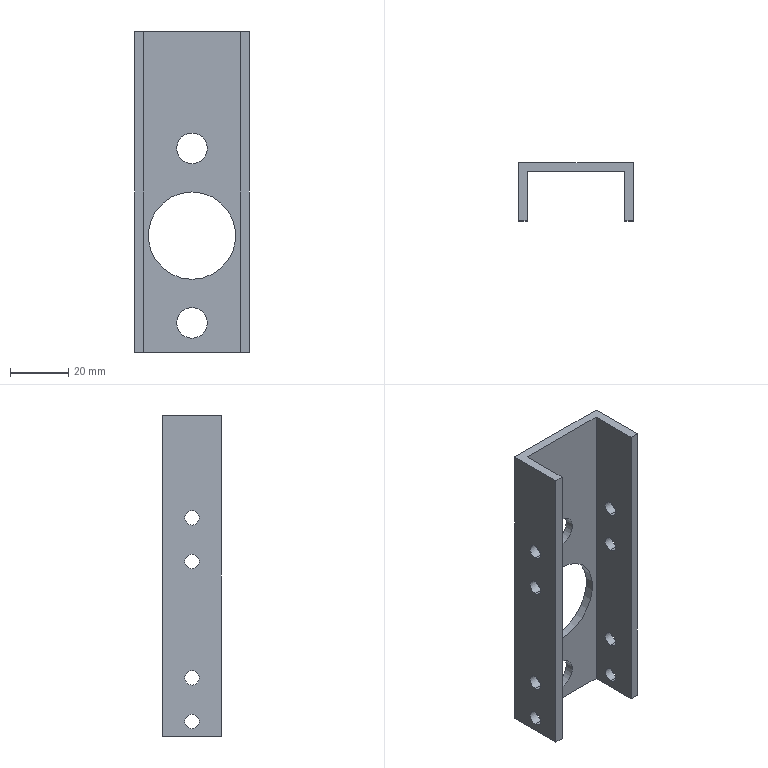Part | SolidWorks | features BaseBody 1 | 1 solid | 32 faces | box 39.5 x 20 x 110 mm | volume 21144 mm3 | cylinder 22 | plane 10 | commonest cylinder face diameters 5 x16 10.5 x4 30 x2
STEP:
#1=CARTESIAN_POINT('',(921.946,-4355.973,909.971));
#2=VERTEX_POINT('',#1);
#3=CARTESIAN_POINT('',(921.946,-4355.973,879.971));
#4=VERTEX_POINT('',#3);
#5=CARTESIAN_POINT('',(921.946,-4355.973,894.971));
#6=DIRECTION('',(0.,-1.,0.));
#7=DIRECTION('',(0.,0.,-1.));
#8=AXIS2_PLACEMENT_3D('',#5,#6,#7);
#9=CIRCLE('',#8,15.);
#10=EDGE_CURVE('',#2,#4,#9,.T.);
#11=ORIENTED_EDGE('',*,*,#10,.F.);
#12=CARTESIAN_POINT('',(921.946,-4358.973,909.971));
#13=VERTEX_POINT('',#12);
#14=CARTESIAN_POINT('',(921.946,-4339.17,909.971));
#15=DIRECTION('',(0.,-1.,0.));
#16=VECTOR('',#15,1000.);
#17=LINE('',#14,#16);
#18=EDGE_CURVE('',#2,#13,#17,.T.);
#19=ORIENTED_EDGE('',*,*,#18,.T.);
#20=CARTESIAN_POINT('',(921.946,-4358.973,879.971));
#21=VERTEX_POINT('',#20);
#22=CARTESIAN_POINT('',(921.946,-4358.973,894.971));
#23=DIRECTION('',(0.,1.,0.));
#24=DIRECTION('',(0.,0.,-1.));
#25=AXIS2_PLACEMENT_3D('',#22,#23,#24);
#26=CIRCLE('',#25,15.);
#27=EDGE_CURVE('',#21,#13,#26,.T.);
#28=ORIENTED_EDGE('',*,*,#27,.F.);
#29=CARTESIAN_POINT('',(921.946,-4339.17,879.971));
#30=DIRECTION('',(0.,-1.,0.));
#31=VECTOR('',#30,1000.);
#32=LINE('',#29,#31);
#33=EDGE_CURVE('',#4,#21,#32,.T.);
#34=ORIENTED_EDGE('',*,*,#33,.F.);
#35=EDGE_LOOP('',(#11,#19,#28,#34));
#36=FACE_OUTER_BOUND('',#35,.T.);
#37=CARTESIAN_POINT('',(921.946,-4339.17,894.971));
#38=DIRECTION('',(0.,-1.,0.));
#39=DIRECTION('',(0.,0.,-1.));
#40=AXIS2_PLACEMENT_3D('',#37,#38,#39);
#41=CYLINDRICAL_SURFACE('',#40,15.);
#42=ADVANCED_FACE('',(#36),#41,.F.);
#43=CARTESIAN_POINT('',(921.946,-4355.973,930.221));
#44=VERTEX_POINT('',#43);
#45=CARTESIAN_POINT('',(921.946,-4355.973,919.721));
#46=VERTEX_POINT('',#45);
#47=CARTESIAN_POINT('',(921.946,-4355.973,924.971));
#48=DIRECTION('',(0.,-1.,0.));
#49=DIRECTION('',(0.,0.,-1.));
#50=AXIS2_PLACEMENT_3D('',#47,#48,#49);
#51=CIRCLE('',#50,5.25);
#52=EDGE_CURVE('',#44,#46,#51,.T.);
#53=ORIENTED_EDGE('',*,*,#52,.F.);
#54=CARTESIAN_POINT('',(921.946,-4358.973,930.221));
#55=VERTEX_POINT('',#54);
#56=CARTESIAN_POINT('',(921.946,-4383.521,930.221));
#57=DIRECTION('',(0.,-1.,0.));
#58=VECTOR('',#57,1000.);
#59=LINE('',#56,#58);
#60=EDGE_CURVE('',#44,#55,#59,.T.);
#61=ORIENTED_EDGE('',*,*,#60,.T.);
#62=CARTESIAN_POINT('',(921.946,-4358.973,919.721));
#63=VERTEX_POINT('',#62);
#64=CARTESIAN_POINT('',(921.946,-4358.973,924.971));
#65=DIRECTION('',(0.,1.,0.));
#66=DIRECTION('',(0.,0.,-1.));
#67=AXIS2_PLACEMENT_3D('',#64,#65,#66);
#68=CIRCLE('',#67,5.25);
#69=EDGE_CURVE('',#63,#55,#68,.T.);
#70=ORIENTED_EDGE('',*,*,#69,.F.);
#71=CARTESIAN_POINT('',(921.946,-4383.521,919.721));
#72=DIRECTION('',(0.,-1.,0.));
#73=VECTOR('',#72,1000.);
#74=LINE('',#71,#73);
#75=EDGE_CURVE('',#46,#63,#74,.T.);
#76=ORIENTED_EDGE('',*,*,#75,.F.);
#77=EDGE_LOOP('',(#53,#61,#70,#76));
#78=FACE_OUTER_BOUND('',#77,.T.);
#79=CARTESIAN_POINT('',(921.946,-4383.521,924.971));
#80=DIRECTION('',(0.,-1.,0.));
#81=DIRECTION('',(0.,0.,-1.));
#82=AXIS2_PLACEMENT_3D('',#79,#80,#81);
#83=CYLINDRICAL_SURFACE('',#82,5.25);
#84=ADVANCED_FACE('',(#78),#83,.F.);
#85=CARTESIAN_POINT('',(921.946,-4358.973,859.721));
#86=VERTEX_POINT('',#85);
#87=CARTESIAN_POINT('',(921.946,-4358.973,870.221));
#88=VERTEX_POINT('',#87);
#89=CARTESIAN_POINT('',(921.946,-4358.973,864.971));
#90=DIRECTION('',(0.,1.,0.));
#91=DIRECTION('',(0.,0.,1.));
#92=AXIS2_PLACEMENT_3D('',#89,#90,#91);
#93=CIRCLE('',#92,5.25);
#94=EDGE_CURVE('',#86,#88,#93,.T.);
#95=ORIENTED_EDGE('',*,*,#94,.F.);
#96=CARTESIAN_POINT('',(921.946,-4355.973,859.721));
#97=VERTEX_POINT('',#96);
#98=CARTESIAN_POINT('',(921.946,-4383.521,859.721));
#99=DIRECTION('',(0.,1.,0.));
#100=VECTOR('',#99,1000.);
#101=LINE('',#98,#100);
#102=EDGE_CURVE('',#86,#97,#101,.T.);
#103=ORIENTED_EDGE('',*,*,#102,.T.);
#104=CARTESIAN_POINT('',(921.946,-4355.973,870.221));
#105=VERTEX_POINT('',#104);
#106=CARTESIAN_POINT('',(921.946,-4355.973,864.971));
#107=DIRECTION('',(0.,-1.,0.));
#108=DIRECTION('',(0.,0.,1.));
#109=AXIS2_PLACEMENT_3D('',#106,#107,#108);
#110=CIRCLE('',#109,5.25);
#111=EDGE_CURVE('',#105,#97,#110,.T.);
#112=ORIENTED_EDGE('',*,*,#111,.F.);
#113=CARTESIAN_POINT('',(921.946,-4383.521,870.221));
#114=DIRECTION('',(0.,1.,0.));
#115=VECTOR('',#114,1000.);
#116=LINE('',#113,#115);
#117=EDGE_CURVE('',#88,#105,#116,.T.);
#118=ORIENTED_EDGE('',*,*,#117,.F.);
#119=EDGE_LOOP('',(#95,#103,#112,#118));
#120=FACE_OUTER_BOUND('',#119,.T.);
#121=CARTESIAN_POINT('',(921.946,-4383.521,864.971));
#122=DIRECTION('',(0.,1.,0.));
#123=DIRECTION('',(0.,0.,1.));
#124=AXIS2_PLACEMENT_3D('',#121,#122,#123);
#125=CYLINDRICAL_SURFACE('',#124,5.25);
#126=ADVANCED_FACE('',(#120),#125,.F.);
#127=CARTESIAN_POINT('',(905.2,-4365.973,927.471));
#128=VERTEX_POINT('',#127);
#129=CARTESIAN_POINT('',(905.2,-4365.973,932.471));
#130=VERTEX_POINT('',#129);
#131=CARTESIAN_POINT('',(905.2,-4365.973,929.971));
#132=DIRECTION('',(-1.,0.,0.));
#133=DIRECTION('',(0.,0.,1.));
#134=AXIS2_PLACEMENT_3D('',#131,#132,#133);
#135=CIRCLE('',#134,2.5);
#136=EDGE_CURVE('',#128,#130,#135,.T.);
#137=ORIENTED_EDGE('',*,*,#136,.F.);
#138=CARTESIAN_POINT('',(902.2,-4365.973,927.471));
#139=VERTEX_POINT('',#138);
#140=CARTESIAN_POINT('',(864.814,-4365.973,927.471));
#141=DIRECTION('',(-1.,0.,0.));
#142=VECTOR('',#141,1000.);
#143=LINE('',#140,#142);
#144=EDGE_CURVE('',#128,#139,#143,.T.);
#145=ORIENTED_EDGE('',*,*,#144,.T.);
#146=CARTESIAN_POINT('',(902.2,-4365.973,932.471));
#147=VERTEX_POINT('',#146);
#148=CARTESIAN_POINT('',(902.2,-4365.973,929.971));
#149=DIRECTION('',(1.,0.,0.));
#150=DIRECTION('',(0.,0.,1.));
#151=AXIS2_PLACEMENT_3D('',#148,#149,#150);
#152=CIRCLE('',#151,2.5);
#153=EDGE_CURVE('',#147,#139,#152,.T.);
#154=ORIENTED_EDGE('',*,*,#153,.F.);
#155=CARTESIAN_POINT('',(864.814,-4365.973,932.471));
#156=DIRECTION('',(-1.,0.,0.));
#157=VECTOR('',#156,1000.);
#158=LINE('',#155,#157);
#159=EDGE_CURVE('',#130,#147,#158,.T.);
#160=ORIENTED_EDGE('',*,*,#159,.F.);
#161=EDGE_LOOP('',(#137,#145,#154,#160));
#162=FACE_OUTER_BOUND('',#161,.T.);
#163=CARTESIAN_POINT('',(864.814,-4365.973,929.971));
#164=DIRECTION('',(-1.,0.,0.));
#165=DIRECTION('',(0.,0.,1.));
#166=AXIS2_PLACEMENT_3D('',#163,#164,#165);
#167=CYLINDRICAL_SURFACE('',#166,2.5);
#168=ADVANCED_FACE('',(#162),#167,.F.);
#169=CARTESIAN_POINT('',(902.2,-4365.973,862.471));
#170=VERTEX_POINT('',#169);
#171=CARTESIAN_POINT('',(902.2,-4365.973,857.471));
#172=VERTEX_POINT('',#171);
#173=CARTESIAN_POINT('',(902.2,-4365.973,859.971));
#174=DIRECTION('',(1.,0.,0.));
#175=DIRECTION('',(0.,0.,-1.));
#176=AXIS2_PLACEMENT_3D('',#173,#174,#175);
#177=CIRCLE('',#176,2.5);
#178=EDGE_CURVE('',#170,#172,#177,.T.);
#179=ORIENTED_EDGE('',*,*,#178,.F.);
#180=CARTESIAN_POINT('',(905.2,-4365.973,862.471));
#181=VERTEX_POINT('',#180);
#182=CARTESIAN_POINT('',(864.814,-4365.973,862.471));
#183=DIRECTION('',(1.,0.,0.));
#184=VECTOR('',#183,1000.);
#185=LINE('',#182,#184);
#186=EDGE_CURVE('',#170,#181,#185,.T.);
#187=ORIENTED_EDGE('',*,*,#186,.T.);
#188=CARTESIAN_POINT('',(905.2,-4365.973,857.471));
#189=VERTEX_POINT('',#188);
#190=CARTESIAN_POINT('',(905.2,-4365.973,859.971));
#191=DIRECTION('',(-1.,0.,0.));
#192=DIRECTION('',(0.,0.,-1.));
#193=AXIS2_PLACEMENT_3D('',#190,#191,#192);
#194=CIRCLE('',#193,2.5);
#195=EDGE_CURVE('',#189,#181,#194,.T.);
#196=ORIENTED_EDGE('',*,*,#195,.F.);
#197=CARTESIAN_POINT('',(864.814,-4365.973,857.471));
#198=DIRECTION('',(1.,0.,0.));
#199=VECTOR('',#198,1000.);
#200=LINE('',#197,#199);
#201=EDGE_CURVE('',#172,#189,#200,.T.);
#202=ORIENTED_EDGE('',*,*,#201,.F.);
#203=EDGE_LOOP('',(#179,#187,#196,#202));
#204=FACE_OUTER_BOUND('',#203,.T.);
#205=CARTESIAN_POINT('',(864.814,-4365.973,859.971));
#206=DIRECTION('',(1.,0.,0.));
#207=DIRECTION('',(0.,0.,-1.));
#208=AXIS2_PLACEMENT_3D('',#205,#206,#207);
#209=CYLINDRICAL_SURFACE('',#208,2.5);
#210=ADVANCED_FACE('',(#204),#209,.F.);
#211=CARTESIAN_POINT('',(902.2,-4365.973,877.471));
#212=VERTEX_POINT('',#211);
#213=CARTESIAN_POINT('',(902.2,-4365.973,872.471));
#214=VERTEX_POINT('',#213);
#215=CARTESIAN_POINT('',(902.2,-4365.973,874.971));
#216=DIRECTION('',(1.,0.,0.));
#217=DIRECTION('',(0.,0.,-1.));
#218=AXIS2_PLACEMENT_3D('',#215,#216,#217);
#219=CIRCLE('',#218,2.5);
#220=EDGE_CURVE('',#212,#214,#219,.T.);
#221=ORIENTED_EDGE('',*,*,#220,.F.);
#222=CARTESIAN_POINT('',(905.2,-4365.973,877.471));
#223=VERTEX_POINT('',#222);
#224=CARTESIAN_POINT('',(864.814,-4365.973,877.471));
#225=DIRECTION('',(1.,0.,0.));
#226=VECTOR('',#225,1000.);
#227=LINE('',#224,#226);
#228=EDGE_CURVE('',#212,#223,#227,.T.);
#229=ORIENTED_EDGE('',*,*,#228,.T.);
#230=CARTESIAN_POINT('',(905.2,-4365.973,872.471));
#231=VERTEX_POINT('',#230);
#232=CARTESIAN_POINT('',(905.2,-4365.973,874.971));
#233=DIRECTION('',(-1.,0.,0.));
#234=DIRECTION('',(0.,0.,-1.));
#235=AXIS2_PLACEMENT_3D('',#232,#233,#234);
#236=CIRCLE('',#235,2.5);
#237=EDGE_CURVE('',#231,#223,#236,.T.);
#238=ORIENTED_EDGE('',*,*,#237,.F.);
#239=CARTESIAN_POINT('',(864.814,-4365.973,872.471));
#240=DIRECTION('',(1.,0.,0.));
#241=VECTOR('',#240,1000.);
#242=LINE('',#239,#241);
#243=EDGE_CURVE('',#214,#231,#242,.T.);
#244=ORIENTED_EDGE('',*,*,#243,.F.);
#245=EDGE_LOOP('',(#221,#229,#238,#244));
#246=FACE_OUTER_BOUND('',#245,.T.);
#247=CARTESIAN_POINT('',(864.814,-4365.973,874.971));
#248=DIRECTION('',(1.,0.,0.));
#249=DIRECTION('',(0.,0.,-1.));
#250=AXIS2_PLACEMENT_3D('',#247,#248,#249);
#251=CYLINDRICAL_SURFACE('',#250,2.5);
#252=ADVANCED_FACE('',(#246),#251,.F.);
#253=CARTESIAN_POINT('',(905.2,-4365.973,912.471));
#254=VERTEX_POINT('',#253);
#255=CARTESIAN_POINT('',(905.2,-4365.973,917.471));
#256=VERTEX_POINT('',#255);
#257=CARTESIAN_POINT('',(905.2,-4365.973,914.971));
#258=DIRECTION('',(-1.,0.,0.));
#259=DIRECTION('',(0.,0.,1.));
#260=AXIS2_PLACEMENT_3D('',#257,#258,#259);
#261=CIRCLE('',#260,2.5);
#262=EDGE_CURVE('',#254,#256,#261,.T.);
#263=ORIENTED_EDGE('',*,*,#262,.F.);
#264=CARTESIAN_POINT('',(902.2,-4365.973,912.471));
#265=VERTEX_POINT('',#264);
#266=CARTESIAN_POINT('',(864.814,-4365.973,912.471));
#267=DIRECTION('',(-1.,0.,0.));
#268=VECTOR('',#267,1000.);
#269=LINE('',#266,#268);
#270=EDGE_CURVE('',#254,#265,#269,.T.);
#271=ORIENTED_EDGE('',*,*,#270,.T.);
#272=CARTESIAN_POINT('',(902.2,-4365.973,917.471));
#273=VERTEX_POINT('',#272);
#274=CARTESIAN_POINT('',(902.2,-4365.973,914.971));
#275=DIRECTION('',(1.,0.,0.));
#276=DIRECTION('',(0.,0.,1.));
#277=AXIS2_PLACEMENT_3D('',#274,#275,#276);
#278=CIRCLE('',#277,2.5);
#279=EDGE_CURVE('',#273,#265,#278,.T.);
#280=ORIENTED_EDGE('',*,*,#279,.F.);
#281=CARTESIAN_POINT('',(864.814,-4365.973,917.471));
#282=DIRECTION('',(-1.,0.,0.));
#283=VECTOR('',#282,1000.);
#284=LINE('',#281,#283);
#285=EDGE_CURVE('',#256,#273,#284,.T.);
#286=ORIENTED_EDGE('',*,*,#285,.F.);
#287=EDGE_LOOP('',(#263,#271,#280,#286));
#288=FACE_OUTER_BOUND('',#287,.T.);
#289=CARTESIAN_POINT('',(864.814,-4365.973,914.971));
#290=DIRECTION('',(-1.,0.,0.));
#291=DIRECTION('',(0.,0.,1.));
#292=AXIS2_PLACEMENT_3D('',#289,#290,#291);
#293=CYLINDRICAL_SURFACE('',#292,2.5);
#294=ADVANCED_FACE('',(#288),#293,.F.);
#295=CARTESIAN_POINT('',(941.7,-4365.973,927.471));
#296=VERTEX_POINT('',#295);
#297=CARTESIAN_POINT('',(941.7,-4365.973,932.471));
#298=VERTEX_POINT('',#297);
#299=CARTESIAN_POINT('',(941.7,-4365.973,929.971));
#300=DIRECTION('',(-1.,0.,0.));
#301=DIRECTION('',(0.,0.,1.));
#302=AXIS2_PLACEMENT_3D('',#299,#300,#301);
#303=CIRCLE('',#302,2.5);
#304=EDGE_CURVE('',#296,#298,#303,.T.);
#305=ORIENTED_EDGE('',*,*,#304,.F.);
#306=CARTESIAN_POINT('',(938.7,-4365.973,927.471));
#307=VERTEX_POINT('',#306);
#308=CARTESIAN_POINT('',(954.922,-4365.973,927.471));
#309=DIRECTION('',(-1.,0.,0.));
#310=VECTOR('',#309,1000.);
#311=LINE('',#308,#310);
#312=EDGE_CURVE('',#296,#307,#311,.T.);
#313=ORIENTED_EDGE('',*,*,#312,.T.);
#314=CARTESIAN_POINT('',(938.7,-4365.973,932.471));
#315=VERTEX_POINT('',#314);
#316=CARTESIAN_POINT('',(938.7,-4365.973,929.971));
#317=DIRECTION('',(1.,0.,0.));
#318=DIRECTION('',(0.,0.,1.));
#319=AXIS2_PLACEMENT_3D('',#316,#317,#318);
#320=CIRCLE('',#319,2.5);
#321=EDGE_CURVE('',#315,#307,#320,.T.);
#322=ORIENTED_EDGE('',*,*,#321,.F.);
#323=CARTESIAN_POINT('',(954.922,-4365.973,932.471));
#324=DIRECTION('',(-1.,0.,0.));
#325=VECTOR('',#324,1000.);
#326=LINE('',#323,#325);
#327=EDGE_CURVE('',#298,#315,#326,.T.);
#328=ORIENTED_EDGE('',*,*,#327,.F.);
#329=EDGE_LOOP('',(#305,#313,#322,#328));
#330=FACE_OUTER_BOUND('',#329,.T.);
#331=CARTESIAN_POINT('',(954.922,-4365.973,929.971));
#332=DIRECTION('',(-1.,0.,0.));
#333=DIRECTION('',(0.,0.,1.));
#334=AXIS2_PLACEMENT_3D('',#331,#332,#333);
#335=CYLINDRICAL_SURFACE('',#334,2.5);
#336=ADVANCED_FACE('',(#330),#335,.F.);
#337=CARTESIAN_POINT('',(938.7,-4365.973,862.471));
#338=VERTEX_POINT('',#337);
#339=CARTESIAN_POINT('',(938.7,-4365.973,857.471));
#340=VERTEX_POINT('',#339);
#341=CARTESIAN_POINT('',(938.7,-4365.973,859.971));
#342=DIRECTION('',(1.,0.,0.));
#343=DIRECTION('',(0.,0.,-1.));
#344=AXIS2_PLACEMENT_3D('',#341,#342,#343);
#345=CIRCLE('',#344,2.5);
#346=EDGE_CURVE('',#338,#340,#345,.T.);
#347=ORIENTED_EDGE('',*,*,#346,.F.);
#348=CARTESIAN_POINT('',(941.7,-4365.973,862.471));
#349=VERTEX_POINT('',#348);
#350=CARTESIAN_POINT('',(954.922,-4365.973,862.471));
#351=DIRECTION('',(1.,0.,0.));
#352=VECTOR('',#351,1000.);
#353=LINE('',#350,#352);
#354=EDGE_CURVE('',#338,#349,#353,.T.);
#355=ORIENTED_EDGE('',*,*,#354,.T.);
#356=CARTESIAN_POINT('',(941.7,-4365.973,857.471));
#357=VERTEX_POINT('',#356);
#358=CARTESIAN_POINT('',(941.7,-4365.973,859.971));
#359=DIRECTION('',(-1.,0.,0.));
#360=DIRECTION('',(0.,0.,-1.));
#361=AXIS2_PLACEMENT_3D('',#358,#359,#360);
#362=CIRCLE('',#361,2.5);
#363=EDGE_CURVE('',#357,#349,#362,.T.);
#364=ORIENTED_EDGE('',*,*,#363,.F.);
#365=CARTESIAN_POINT('',(954.922,-4365.973,857.471));
#366=DIRECTION('',(1.,0.,0.));
#367=VECTOR('',#366,1000.);
#368=LINE('',#365,#367);
#369=EDGE_CURVE('',#340,#357,#368,.T.);
#370=ORIENTED_EDGE('',*,*,#369,.F.);
#371=EDGE_LOOP('',(#347,#355,#364,#370));
#372=FACE_OUTER_BOUND('',#371,.T.);
#373=CARTESIAN_POINT('',(954.922,-4365.973,859.971));
#374=DIRECTION('',(1.,0.,0.));
#375=DIRECTION('',(0.,0.,-1.));
#376=AXIS2_PLACEMENT_3D('',#373,#374,#375);
#377=CYLINDRICAL_SURFACE('',#376,2.5);
#378=ADVANCED_FACE('',(#372),#377,.F.);
#379=CARTESIAN_POINT('',(938.7,-4365.973,877.471));
#380=VERTEX_POINT('',#379);
#381=CARTESIAN_POINT('',(938.7,-4365.973,872.471));
#382=VERTEX_POINT('',#381);
#383=CARTESIAN_POINT('',(938.7,-4365.973,874.971));
#384=DIRECTION('',(1.,0.,0.));
#385=DIRECTION('',(0.,0.,-1.));
#386=AXIS2_PLACEMENT_3D('',#383,#384,#385);
#387=CIRCLE('',#386,2.5);
#388=EDGE_CURVE('',#380,#382,#387,.T.);
#389=ORIENTED_EDGE('',*,*,#388,.F.);
#390=CARTESIAN_POINT('',(941.7,-4365.973,877.471));
#391=VERTEX_POINT('',#390);
#392=CARTESIAN_POINT('',(954.922,-4365.973,877.471));
#393=DIRECTION('',(1.,0.,0.));
#394=VECTOR('',#393,1000.);
#395=LINE('',#392,#394);
#396=EDGE_CURVE('',#380,#391,#395,.T.);
#397=ORIENTED_EDGE('',*,*,#396,.T.);
#398=CARTESIAN_POINT('',(941.7,-4365.973,872.471));
#399=VERTEX_POINT('',#398);
#400=CARTESIAN_POINT('',(941.7,-4365.973,874.971));
#401=DIRECTION('',(-1.,0.,0.));
#402=DIRECTION('',(0.,0.,-1.));
#403=AXIS2_PLACEMENT_3D('',#400,#401,#402);
#404=CIRCLE('',#403,2.5);
#405=EDGE_CURVE('',#399,#391,#404,.T.);
#406=ORIENTED_EDGE('',*,*,#405,.F.);
#407=CARTESIAN_POINT('',(954.922,-4365.973,872.471));
#408=DIRECTION('',(1.,0.,0.));
#409=VECTOR('',#408,1000.);
#410=LINE('',#407,#409);
#411=EDGE_CURVE('',#382,#399,#410,.T.);
#412=ORIENTED_EDGE('',*,*,#411,.F.);
#413=EDGE_LOOP('',(#389,#397,#406,#412));
#414=FACE_OUTER_BOUND('',#413,.T.);
#415=CARTESIAN_POINT('',(954.922,-4365.973,874.971));
#416=DIRECTION('',(1.,0.,0.));
#417=DIRECTION('',(0.,0.,-1.));
#418=AXIS2_PLACEMENT_3D('',#415,#416,#417);
#419=CYLINDRICAL_SURFACE('',#418,2.5);
#420=ADVANCED_FACE('',(#414),#419,.F.);
#421=CARTESIAN_POINT('',(941.7,-4365.973,912.471));
#422=VERTEX_POINT('',#421);
#423=CARTESIAN_POINT('',(941.7,-4365.973,917.471));
#424=VERTEX_POINT('',#423);
#425=CARTESIAN_POINT('',(941.7,-4365.973,914.971));
#426=DIRECTION('',(-1.,0.,0.));
#427=DIRECTION('',(0.,0.,1.));
#428=AXIS2_PLACEMENT_3D('',#425,#426,#427);
#429=CIRCLE('',#428,2.5);
#430=EDGE_CURVE('',#422,#424,#429,.T.);
#431=ORIENTED_EDGE('',*,*,#430,.F.);
#432=CARTESIAN_POINT('',(938.7,-4365.973,912.471));
#433=VERTEX_POINT('',#432);
#434=CARTESIAN_POINT('',(954.922,-4365.973,912.471));
#435=DIRECTION('',(-1.,0.,0.));
#436=VECTOR('',#435,1000.);
#437=LINE('',#434,#436);
#438=EDGE_CURVE('',#422,#433,#437,.T.);
#439=ORIENTED_EDGE('',*,*,#438,.T.);
#440=CARTESIAN_POINT('',(938.7,-4365.973,917.471));
#441=VERTEX_POINT('',#440);
#442=CARTESIAN_POINT('',(938.7,-4365.973,914.971));
#443=DIRECTION('',(1.,0.,0.));
#444=DIRECTION('',(0.,0.,1.));
#445=AXIS2_PLACEMENT_3D('',#442,#443,#444);
#446=CIRCLE('',#445,2.5);
#447=EDGE_CURVE('',#441,#433,#446,.T.);
#448=ORIENTED_EDGE('',*,*,#447,.F.);
#449=CARTESIAN_POINT('',(954.922,-4365.973,917.471));
#450=DIRECTION('',(-1.,0.,0.));
#451=VECTOR('',#450,1000.);
#452=LINE('',#449,#451);
#453=EDGE_CURVE('',#424,#441,#452,.T.);
#454=ORIENTED_EDGE('',*,*,#453,.F.);
#455=EDGE_LOOP('',(#431,#439,#448,#454));
#456=FACE_OUTER_BOUND('',#455,.T.);
#457=CARTESIAN_POINT('',(954.922,-4365.973,914.971));
#458=DIRECTION('',(-1.,0.,0.));
#459=DIRECTION('',(0.,0.,1.));
#460=AXIS2_PLACEMENT_3D('',#457,#458,#459);
#461=CYLINDRICAL_SURFACE('',#460,2.5);
#462=ADVANCED_FACE('',(#456),#461,.F.);
#463=CARTESIAN_POINT('',(941.7,-4355.973,854.971));
#464=VERTEX_POINT('',#463);
#465=CARTESIAN_POINT('',(902.2,-4355.973,854.971));
#466=VERTEX_POINT('',#465);
#467=CARTESIAN_POINT('',(941.7,-4355.973,854.971));
#468=DIRECTION('',(-1.,0.,0.));
#469=VECTOR('',#468,1000.);
#470=LINE('',#467,#469);
#471=EDGE_CURVE('',#464,#466,#470,.T.);
#472=ORIENTED_EDGE('',*,*,#471,.T.);
#473=CARTESIAN_POINT('',(902.2,-4355.973,964.971));
#474=VERTEX_POINT('',#473);
#475=CARTESIAN_POINT('',(902.2,-4355.973,854.971));
#476=DIRECTION('',(0.,0.,1.));
#477=VECTOR('',#476,1000.);
#478=LINE('',#475,#477);
#479=EDGE_CURVE('',#466,#474,#478,.T.);
#480=ORIENTED_EDGE('',*,*,#479,.T.);
#481=CARTESIAN_POINT('',(941.7,-4355.973,964.971));
#482=VERTEX_POINT('',#481);
#483=CARTESIAN_POINT('',(941.7,-4355.973,964.971));
#484=DIRECTION('',(1.,0.,0.));
#485=VECTOR('',#484,1000.);
#486=LINE('',#483,#485);
#487=EDGE_CURVE('',#474,#482,#486,.T.);
#488=ORIENTED_EDGE('',*,*,#487,.T.);
#489=CARTESIAN_POINT('',(941.7,-4355.973,854.971));
#490=DIRECTION('',(0.,0.,-1.));
#491=VECTOR('',#490,1000.);
#492=LINE('',#489,#491);
#493=EDGE_CURVE('',#482,#464,#492,.T.);
#494=ORIENTED_EDGE('',*,*,#493,.T.);
#495=EDGE_LOOP('',(#472,#480,#488,#494));
#496=FACE_OUTER_BOUND('',#495,.T.);
#497=CARTESIAN_POINT('',(921.946,-4355.973,894.971));
#498=DIRECTION('',(0.,-1.,0.));
#499=DIRECTION('',(0.,0.,-1.));
#500=AXIS2_PLACEMENT_3D('',#497,#498,#499);
#501=CIRCLE('',#500,15.);
#502=EDGE_CURVE('',#4,#2,#501,.T.);
#503=ORIENTED_EDGE('',*,*,#502,.T.);
#504=ORIENTED_EDGE('',*,*,#10,.T.);
#505=EDGE_LOOP('',(#503,#504));
#506=FACE_BOUND('',#505,.T.);
#507=CARTESIAN_POINT('',(921.946,-4355.973,924.971));
#508=DIRECTION('',(0.,-1.,0.));
#509=DIRECTION('',(0.,0.,-1.));
#510=AXIS2_PLACEMENT_3D('',#507,#508,#509);
#511=CIRCLE('',#510,5.25);
#512=EDGE_CURVE('',#46,#44,#511,.T.);
#513=ORIENTED_EDGE('',*,*,#512,.T.);
#514=ORIENTED_EDGE('',*,*,#52,.T.);
#515=EDGE_LOOP('',(#513,#514));
#516=FACE_BOUND('',#515,.T.);
#517=ORIENTED_EDGE('',*,*,#111,.T.);
#518=CARTESIAN_POINT('',(921.946,-4355.973,864.971));
#519=DIRECTION('',(0.,-1.,0.));
#520=DIRECTION('',(0.,0.,1.));
#521=AXIS2_PLACEMENT_3D('',#518,#519,#520);
#522=CIRCLE('',#521,5.25);
#523=EDGE_CURVE('',#97,#105,#522,.T.);
#524=ORIENTED_EDGE('',*,*,#523,.T.);
#525=EDGE_LOOP('',(#517,#524));
#526=FACE_BOUND('',#525,.T.);
#527=CARTESIAN_POINT('',(941.7,-4355.973,854.971));
#528=DIRECTION('',(0.,1.,0.));
#529=DIRECTION('',(0.,0.,1.));
#530=AXIS2_PLACEMENT_3D('',#527,#528,#529);
#531=PLANE('',#530);
#532=ADVANCED_FACE('',(#496,#506,#516,#526),#531,.T.);
#533=CARTESIAN_POINT('',(902.2,-4375.973,854.971));
#534=VERTEX_POINT('',#533);
#535=CARTESIAN_POINT('',(902.2,-4345.973,854.971));
#536=DIRECTION('',(0.,-1.,0.));
#537=VECTOR('',#536,1000.);
#538=LINE('',#535,#537);
#539=EDGE_CURVE('',#466,#534,#538,.T.);
#540=ORIENTED_EDGE('',*,*,#539,.T.);
#541=CARTESIAN_POINT('',(902.2,-4375.973,964.971));
#542=VERTEX_POINT('',#541);
#543=CARTESIAN_POINT('',(902.2,-4375.973,854.971));
#544=DIRECTION('',(0.,0.,1.));
#545=VECTOR('',#544,1000.);
#546=LINE('',#543,#545);
#547=EDGE_CURVE('',#534,#542,#546,.T.);
#548=ORIENTED_EDGE('',*,*,#547,.T.);
#549=CARTESIAN_POINT('',(902.2,-4345.973,964.971));
#550=DIRECTION('',(0.,1.,0.));
#551=VECTOR('',#550,1000.);
#552=LINE('',#549,#551);
#553=EDGE_CURVE('',#542,#474,#552,.T.);
#554=ORIENTED_EDGE('',*,*,#553,.T.);
#555=ORIENTED_EDGE('',*,*,#479,.F.);
#556=EDGE_LOOP('',(#540,#548,#554,#555));
#557=FACE_OUTER_BOUND('',#556,.T.);
#558=ORIENTED_EDGE('',*,*,#153,.T.);
#559=CARTESIAN_POINT('',(902.2,-4365.973,929.971));
#560=DIRECTION('',(1.,0.,0.));
#561=DIRECTION('',(0.,0.,1.));
#562=AXIS2_PLACEMENT_3D('',#559,#560,#561);
#563=CIRCLE('',#562,2.5);
#564=EDGE_CURVE('',#139,#147,#563,.T.);
#565=ORIENTED_EDGE('',*,*,#564,.T.);
#566=EDGE_LOOP('',(#558,#565));
#567=FACE_BOUND('',#566,.T.);
#568=CARTESIAN_POINT('',(902.2,-4365.973,859.971));
#569=DIRECTION('',(1.,0.,0.));
#570=DIRECTION('',(0.,0.,-1.));
#571=AXIS2_PLACEMENT_3D('',#568,#569,#570);
#572=CIRCLE('',#571,2.5);
#573=EDGE_CURVE('',#172,#170,#572,.T.);
#574=ORIENTED_EDGE('',*,*,#573,.T.);
#575=ORIENTED_EDGE('',*,*,#178,.T.);
#576=EDGE_LOOP('',(#574,#575));
#577=FACE_BOUND('',#576,.T.);
#578=CARTESIAN_POINT('',(902.2,-4365.973,874.971));
#579=DIRECTION('',(1.,0.,0.));
#580=DIRECTION('',(0.,0.,-1.));
#581=AXIS2_PLACEMENT_3D('',#578,#579,#580);
#582=CIRCLE('',#581,2.5);
#583=EDGE_CURVE('',#214,#212,#582,.T.);
#584=ORIENTED_EDGE('',*,*,#583,.T.);
#585=ORIENTED_EDGE('',*,*,#220,.T.);
#586=EDGE_LOOP('',(#584,#585));
#587=FACE_BOUND('',#586,.T.);
#588=ORIENTED_EDGE('',*,*,#279,.T.);
#589=CARTESIAN_POINT('',(902.2,-4365.973,914.971));
#590=DIRECTION('',(1.,0.,0.));
#591=DIRECTION('',(0.,0.,1.));
#592=AXIS2_PLACEMENT_3D('',#589,#590,#591);
#593=CIRCLE('',#592,2.5);
#594=EDGE_CURVE('',#265,#273,#593,.T.);
#595=ORIENTED_EDGE('',*,*,#594,.T.);
#596=EDGE_LOOP('',(#588,#595));
#597=FACE_BOUND('',#596,.T.);
#598=CARTESIAN_POINT('',(902.2,-4345.973,854.971));
#599=DIRECTION('',(-1.,0.,0.));
#600=DIRECTION('',(0.,0.,1.));
#601=AXIS2_PLACEMENT_3D('',#598,#599,#600);
#602=PLANE('',#601);
#603=ADVANCED_FACE('',(#557,#567,#577,#587,#597),#602,.T.);
#604=CARTESIAN_POINT('',(905.2,-4375.973,854.971));
#605=VERTEX_POINT('',#604);
#606=CARTESIAN_POINT('',(905.2,-4358.973,854.971));
#607=VERTEX_POINT('',#606);
#608=CARTESIAN_POINT('',(905.2,-4356.706,854.971));
#609=DIRECTION('',(0.,1.,0.));
#610=VECTOR('',#609,1000.);
#611=LINE('',#608,#610);
#612=EDGE_CURVE('',#605,#607,#611,.T.);
#613=ORIENTED_EDGE('',*,*,#612,.F.);
#614=CARTESIAN_POINT('',(921.95,-4375.973,854.971));
#615=DIRECTION('',(1.,0.,0.));
#616=VECTOR('',#615,1000.);
#617=LINE('',#614,#616);
#618=EDGE_CURVE('',#534,#605,#617,.T.);
#619=ORIENTED_EDGE('',*,*,#618,.F.);
#620=ORIENTED_EDGE('',*,*,#539,.F.);
#621=ORIENTED_EDGE('',*,*,#471,.F.);
#622=CARTESIAN_POINT('',(941.7,-4375.973,854.971));
#623=VERTEX_POINT('',#622);
#624=CARTESIAN_POINT('',(941.7,-4356.706,854.971));
#625=DIRECTION('',(0.,1.,0.));
#626=VECTOR('',#625,1000.);
#627=LINE('',#624,#626);
#628=EDGE_CURVE('',#623,#464,#627,.T.);
#629=ORIENTED_EDGE('',*,*,#628,.F.);
#630=CARTESIAN_POINT('',(938.7,-4375.973,854.971));
#631=VERTEX_POINT('',#630);
#632=CARTESIAN_POINT('',(921.95,-4375.973,854.971));
#633=DIRECTION('',(1.,0.,0.));
#634=VECTOR('',#633,1000.);
#635=LINE('',#632,#634);
#636=EDGE_CURVE('',#631,#623,#635,.T.);
#637=ORIENTED_EDGE('',*,*,#636,.F.);
#638=CARTESIAN_POINT('',(938.7,-4358.973,854.971));
#639=VERTEX_POINT('',#638);
#640=CARTESIAN_POINT('',(938.7,-4356.706,854.971));
#641=DIRECTION('',(0.,-1.,0.));
#642=VECTOR('',#641,1000.);
#643=LINE('',#640,#642);
#644=EDGE_CURVE('',#639,#631,#643,.T.);
#645=ORIENTED_EDGE('',*,*,#644,.F.);
#646=CARTESIAN_POINT('',(921.95,-4358.973,854.971));
#647=DIRECTION('',(1.,0.,0.));
#648=VECTOR('',#647,1000.);
#649=LINE('',#646,#648);
#650=EDGE_CURVE('',#607,#639,#649,.T.);
#651=ORIENTED_EDGE('',*,*,#650,.F.);
#652=EDGE_LOOP('',(#613,#619,#620,#621,#629,#637,#645,#651));
#653=FACE_OUTER_BOUND('',#652,.T.);
#654=CARTESIAN_POINT('',(921.95,-4356.706,854.971));
#655=DIRECTION('',(0.,0.,1.));
#656=DIRECTION('',(1.,0.,0.));
#657=AXIS2_PLACEMENT_3D('',#654,#655,#656);
#658=PLANE('',#657);
#659=ADVANCED_FACE('',(#653),#658,.F.);
#660=ORIENTED_EDGE('',*,*,#628,.T.);
#661=ORIENTED_EDGE('',*,*,#493,.F.);
#662=CARTESIAN_POINT('',(941.7,-4375.973,964.971));
#663=VERTEX_POINT('',#662);
#664=CARTESIAN_POINT('',(941.7,-4375.973,964.971));
#665=DIRECTION('',(0.,-1.,0.));
#666=VECTOR('',#665,1000.);
#667=LINE('',#664,#666);
#668=EDGE_CURVE('',#482,#663,#667,.T.);
#669=ORIENTED_EDGE('',*,*,#668,.T.);
#670=CARTESIAN_POINT('',(941.7,-4375.973,854.971));
#671=DIRECTION('',(0.,0.,-1.));
#672=VECTOR('',#671,1000.);
#673=LINE('',#670,#672);
#674=EDGE_CURVE('',#663,#623,#673,.T.);
#675=ORIENTED_EDGE('',*,*,#674,.T.);
#676=EDGE_LOOP('',(#660,#661,#669,#675));
#677=FACE_OUTER_BOUND('',#676,.T.);
#678=CARTESIAN_POINT('',(941.7,-4365.973,929.971));
#679=DIRECTION('',(-1.,0.,0.));
#680=DIRECTION('',(0.,0.,1.));
#681=AXIS2_PLACEMENT_3D('',#678,#679,#680);
#682=CIRCLE('',#681,2.5);
#683=EDGE_CURVE('',#298,#296,#682,.T.);
#684=ORIENTED_EDGE('',*,*,#683,.T.);
#685=ORIENTED_EDGE('',*,*,#304,.T.);
#686=EDGE_LOOP('',(#684,#685));
#687=FACE_BOUND('',#686,.T.);
#688=ORIENTED_EDGE('',*,*,#363,.T.);
#689=CARTESIAN_POINT('',(941.7,-4365.973,859.971));
#690=DIRECTION('',(-1.,0.,0.));
#691=DIRECTION('',(0.,0.,-1.));
#692=AXIS2_PLACEMENT_3D('',#689,#690,#691);
#693=CIRCLE('',#692,2.5);
#694=EDGE_CURVE('',#349,#357,#693,.T.);
#695=ORIENTED_EDGE('',*,*,#694,.T.);
#696=EDGE_LOOP('',(#688,#695));
#697=FACE_BOUND('',#696,.T.);
#698=ORIENTED_EDGE('',*,*,#405,.T.);
#699=CARTESIAN_POINT('',(941.7,-4365.973,874.971));
#700=DIRECTION('',(-1.,0.,0.));
#701=DIRECTION('',(0.,0.,-1.));
#702=AXIS2_PLACEMENT_3D('',#699,#700,#701);
#703=CIRCLE('',#702,2.5);
#704=EDGE_CURVE('',#391,#399,#703,.T.);
#705=ORIENTED_EDGE('',*,*,#704,.T.);
#706=EDGE_LOOP('',(#698,#705));
#707=FACE_BOUND('',#706,.T.);
#708=CARTESIAN_POINT('',(941.7,-4365.973,914.971));
#709=DIRECTION('',(-1.,0.,0.));
#710=DIRECTION('',(0.,0.,1.));
#711=AXIS2_PLACEMENT_3D('',#708,#709,#710);
#712=CIRCLE('',#711,2.5);
#713=EDGE_CURVE('',#424,#422,#712,.T.);
#714=ORIENTED_EDGE('',*,*,#713,.T.);
#715=ORIENTED_EDGE('',*,*,#430,.T.);
#716=EDGE_LOOP('',(#714,#715));
#717=FACE_BOUND('',#716,.T.);
#718=CARTESIAN_POINT('',(941.7,-4375.973,854.971));
#719=DIRECTION('',(1.,0.,0.));
#720=DIRECTION('',(0.,0.,-1.));
#721=AXIS2_PLACEMENT_3D('',#718,#719,#720);
#722=PLANE('',#721);
#723=ADVANCED_FACE('',(#677,#687,#697,#707,#717),#722,.T.);
#724=CARTESIAN_POINT('',(905.2,-4375.973,964.971));
#725=VERTEX_POINT('',#724);
#726=CARTESIAN_POINT('',(905.2,-4358.973,964.971));
#727=VERTEX_POINT('',#726);
#728=CARTESIAN_POINT('',(905.2,-4356.706,964.971));
#729=DIRECTION('',(0.,1.,0.));
#730=VECTOR('',#729,1000.);
#731=LINE('',#728,#730);
#732=EDGE_CURVE('',#725,#727,#731,.T.);
#733=ORIENTED_EDGE('',*,*,#732,.T.);
#734=CARTESIAN_POINT('',(938.7,-4358.973,964.971));
#735=VERTEX_POINT('',#734);
#736=CARTESIAN_POINT('',(921.95,-4358.973,964.971));
#737=DIRECTION('',(1.,0.,0.));
#738=VECTOR('',#737,1000.);
#739=LINE('',#736,#738);
#740=EDGE_CURVE('',#727,#735,#739,.T.);
#741=ORIENTED_EDGE('',*,*,#740,.T.);
#742=CARTESIAN_POINT('',(938.7,-4375.973,964.971));
#743=VERTEX_POINT('',#742);
#744=CARTESIAN_POINT('',(938.7,-4356.706,964.971));
#745=DIRECTION('',(0.,-1.,0.));
#746=VECTOR('',#745,1000.);
#747=LINE('',#744,#746);
#748=EDGE_CURVE('',#735,#743,#747,.T.);
#749=ORIENTED_EDGE('',*,*,#748,.T.);
#750=CARTESIAN_POINT('',(921.95,-4375.973,964.971));
#751=DIRECTION('',(1.,0.,0.));
#752=VECTOR('',#751,1000.);
#753=LINE('',#750,#752);
#754=EDGE_CURVE('',#743,#663,#753,.T.);
#755=ORIENTED_EDGE('',*,*,#754,.T.);
#756=ORIENTED_EDGE('',*,*,#668,.F.);
#757=ORIENTED_EDGE('',*,*,#487,.F.);
#758=ORIENTED_EDGE('',*,*,#553,.F.);
#759=CARTESIAN_POINT('',(921.95,-4375.973,964.971));
#760=DIRECTION('',(1.,0.,0.));
#761=VECTOR('',#760,1000.);
#762=LINE('',#759,#761);
#763=EDGE_CURVE('',#542,#725,#762,.T.);
#764=ORIENTED_EDGE('',*,*,#763,.T.);
#765=EDGE_LOOP('',(#733,#741,#749,#755,#756,#757,#758,#764));
#766=FACE_OUTER_BOUND('',#765,.T.);
#767=CARTESIAN_POINT('',(921.95,-4356.706,964.971));
#768=DIRECTION('',(0.,0.,1.));
#769=DIRECTION('',(1.,0.,0.));
#770=AXIS2_PLACEMENT_3D('',#767,#768,#769);
#771=PLANE('',#770);
#772=ADVANCED_FACE('',(#766),#771,.T.);
#773=ORIENTED_EDGE('',*,*,#18,.F.);
#774=ORIENTED_EDGE('',*,*,#502,.F.);
#775=ORIENTED_EDGE('',*,*,#33,.T.);
#776=CARTESIAN_POINT('',(921.946,-4358.973,894.971));
#777=DIRECTION('',(0.,1.,0.));
#778=DIRECTION('',(0.,0.,-1.));
#779=AXIS2_PLACEMENT_3D('',#776,#777,#778);
#780=CIRCLE('',#779,15.);
#781=EDGE_CURVE('',#13,#21,#780,.T.);
#782=ORIENTED_EDGE('',*,*,#781,.F.);
#783=EDGE_LOOP('',(#773,#774,#775,#782));
#784=FACE_OUTER_BOUND('',#783,.T.);
#785=CARTESIAN_POINT('',(921.946,-4339.17,894.971));
#786=DIRECTION('',(0.,-1.,0.));
#787=DIRECTION('',(0.,0.,-1.));
#788=AXIS2_PLACEMENT_3D('',#785,#786,#787);
#789=CYLINDRICAL_SURFACE('',#788,15.);
#790=ADVANCED_FACE('',(#784),#789,.F.);
#791=ORIENTED_EDGE('',*,*,#60,.F.);
#792=ORIENTED_EDGE('',*,*,#512,.F.);
#793=ORIENTED_EDGE('',*,*,#75,.T.);
#794=CARTESIAN_POINT('',(921.946,-4358.973,924.971));
#795=DIRECTION('',(0.,1.,0.));
#796=DIRECTION('',(0.,0.,-1.));
#797=AXIS2_PLACEMENT_3D('',#794,#795,#796);
#798=CIRCLE('',#797,5.25);
#799=EDGE_CURVE('',#55,#63,#798,.T.);
#800=ORIENTED_EDGE('',*,*,#799,.F.);
#801=EDGE_LOOP('',(#791,#792,#793,#800));
#802=FACE_OUTER_BOUND('',#801,.T.);
#803=CARTESIAN_POINT('',(921.946,-4383.521,924.971));
#804=DIRECTION('',(0.,-1.,0.));
#805=DIRECTION('',(0.,0.,-1.));
#806=AXIS2_PLACEMENT_3D('',#803,#804,#805);
#807=CYLINDRICAL_SURFACE('',#806,5.25);
#808=ADVANCED_FACE('',(#802),#807,.F.);
#809=ORIENTED_EDGE('',*,*,#102,.F.);
#810=CARTESIAN_POINT('',(921.946,-4358.973,864.971));
#811=DIRECTION('',(0.,1.,0.));
#812=DIRECTION('',(0.,0.,1.));
#813=AXIS2_PLACEMENT_3D('',#810,#811,#812);
#814=CIRCLE('',#813,5.25);
#815=EDGE_CURVE('',#88,#86,#814,.T.);
#816=ORIENTED_EDGE('',*,*,#815,.F.);
#817=ORIENTED_EDGE('',*,*,#117,.T.);
#818=ORIENTED_EDGE('',*,*,#523,.F.);
#819=EDGE_LOOP('',(#809,#816,#817,#818));
#820=FACE_OUTER_BOUND('',#819,.T.);
#821=CARTESIAN_POINT('',(921.946,-4383.521,864.971));
#822=DIRECTION('',(0.,1.,0.));
#823=DIRECTION('',(0.,0.,1.));
#824=AXIS2_PLACEMENT_3D('',#821,#822,#823);
#825=CYLINDRICAL_SURFACE('',#824,5.25);
#826=ADVANCED_FACE('',(#820),#825,.F.);
#827=ORIENTED_EDGE('',*,*,#618,.T.);
#828=CARTESIAN_POINT('',(905.2,-4375.973,854.971));
#829=DIRECTION('',(0.,0.,1.));
#830=VECTOR('',#829,1000.);
#831=LINE('',#828,#830);
#832=EDGE_CURVE('',#605,#725,#831,.T.);
#833=ORIENTED_EDGE('',*,*,#832,.T.);
#834=ORIENTED_EDGE('',*,*,#763,.F.);
#835=ORIENTED_EDGE('',*,*,#547,.F.);
#836=EDGE_LOOP('',(#827,#833,#834,#835));
#837=FACE_OUTER_BOUND('',#836,.T.);
#838=CARTESIAN_POINT('',(902.2,-4375.973,854.971));
#839=DIRECTION('',(0.,-1.,0.));
#840=DIRECTION('',(0.,0.,-1.));
#841=AXIS2_PLACEMENT_3D('',#838,#839,#840);
#842=PLANE('',#841);
#843=ADVANCED_FACE('',(#837),#842,.T.);
#844=ORIENTED_EDGE('',*,*,#144,.F.);
#845=CARTESIAN_POINT('',(905.2,-4365.973,929.971));
#846=DIRECTION('',(-1.,0.,0.));
#847=DIRECTION('',(0.,0.,1.));
#848=AXIS2_PLACEMENT_3D('',#845,#846,#847);
#849=CIRCLE('',#848,2.5);
#850=EDGE_CURVE('',#130,#128,#849,.T.);
#851=ORIENTED_EDGE('',*,*,#850,.F.);
#852=ORIENTED_EDGE('',*,*,#159,.T.);
#853=ORIENTED_EDGE('',*,*,#564,.F.);
#854=EDGE_LOOP('',(#844,#851,#852,#853));
#855=FACE_OUTER_BOUND('',#854,.T.);
#856=CARTESIAN_POINT('',(864.814,-4365.973,929.971));
#857=DIRECTION('',(-1.,0.,0.));
#858=DIRECTION('',(0.,0.,1.));
#859=AXIS2_PLACEMENT_3D('',#856,#857,#858);
#860=CYLINDRICAL_SURFACE('',#859,2.5);
#861=ADVANCED_FACE('',(#855),#860,.F.);
#862=ORIENTED_EDGE('',*,*,#186,.F.);
#863=ORIENTED_EDGE('',*,*,#573,.F.);
#864=ORIENTED_EDGE('',*,*,#201,.T.);
#865=CARTESIAN_POINT('',(905.2,-4365.973,859.971));
#866=DIRECTION('',(-1.,0.,0.));
#867=DIRECTION('',(0.,0.,-1.));
#868=AXIS2_PLACEMENT_3D('',#865,#866,#867);
#869=CIRCLE('',#868,2.5);
#870=EDGE_CURVE('',#181,#189,#869,.T.);
#871=ORIENTED_EDGE('',*,*,#870,.F.);
#872=EDGE_LOOP('',(#862,#863,#864,#871));
#873=FACE_OUTER_BOUND('',#872,.T.);
#874=CARTESIAN_POINT('',(864.814,-4365.973,859.971));
#875=DIRECTION('',(1.,0.,0.));
#876=DIRECTION('',(0.,0.,-1.));
#877=AXIS2_PLACEMENT_3D('',#874,#875,#876);
#878=CYLINDRICAL_SURFACE('',#877,2.5);
#879=ADVANCED_FACE('',(#873),#878,.F.);
#880=ORIENTED_EDGE('',*,*,#228,.F.);
#881=ORIENTED_EDGE('',*,*,#583,.F.);
#882=ORIENTED_EDGE('',*,*,#243,.T.);
#883=CARTESIAN_POINT('',(905.2,-4365.973,874.971));
#884=DIRECTION('',(-1.,0.,0.));
#885=DIRECTION('',(0.,0.,-1.));
#886=AXIS2_PLACEMENT_3D('',#883,#884,#885);
#887=CIRCLE('',#886,2.5);
#888=EDGE_CURVE('',#223,#231,#887,.T.);
#889=ORIENTED_EDGE('',*,*,#888,.F.);
#890=EDGE_LOOP('',(#880,#881,#882,#889));
#891=FACE_OUTER_BOUND('',#890,.T.);
#892=CARTESIAN_POINT('',(864.814,-4365.973,874.971));
#893=DIRECTION('',(1.,0.,0.));
#894=DIRECTION('',(0.,0.,-1.));
#895=AXIS2_PLACEMENT_3D('',#892,#893,#894);
#896=CYLINDRICAL_SURFACE('',#895,2.5);
#897=ADVANCED_FACE('',(#891),#896,.F.);
#898=ORIENTED_EDGE('',*,*,#270,.F.);
#899=CARTESIAN_POINT('',(905.2,-4365.973,914.971));
#900=DIRECTION('',(-1.,0.,0.));
#901=DIRECTION('',(0.,0.,1.));
#902=AXIS2_PLACEMENT_3D('',#899,#900,#901);
#903=CIRCLE('',#902,2.5);
#904=EDGE_CURVE('',#256,#254,#903,.T.);
#905=ORIENTED_EDGE('',*,*,#904,.F.);
#906=ORIENTED_EDGE('',*,*,#285,.T.);
#907=ORIENTED_EDGE('',*,*,#594,.F.);
#908=EDGE_LOOP('',(#898,#905,#906,#907));
#909=FACE_OUTER_BOUND('',#908,.T.);
#910=CARTESIAN_POINT('',(864.814,-4365.973,914.971));
#911=DIRECTION('',(-1.,0.,0.));
#912=DIRECTION('',(0.,0.,1.));
#913=AXIS2_PLACEMENT_3D('',#910,#911,#912);
#914=CYLINDRICAL_SURFACE('',#913,2.5);
#915=ADVANCED_FACE('',(#909),#914,.F.);
#916=ORIENTED_EDGE('',*,*,#650,.T.);
#917=CARTESIAN_POINT('',(938.7,-4358.973,854.971));
#918=DIRECTION('',(0.,0.,1.));
#919=VECTOR('',#918,1000.);
#920=LINE('',#917,#919);
#921=EDGE_CURVE('',#639,#735,#920,.T.);
#922=ORIENTED_EDGE('',*,*,#921,.T.);
#923=ORIENTED_EDGE('',*,*,#740,.F.);
#924=CARTESIAN_POINT('',(905.2,-4358.973,854.971));
#925=DIRECTION('',(0.,0.,-1.));
#926=VECTOR('',#925,1000.);
#927=LINE('',#924,#926);
#928=EDGE_CURVE('',#727,#607,#927,.T.);
#929=ORIENTED_EDGE('',*,*,#928,.T.);
#930=EDGE_LOOP('',(#916,#922,#923,#929));
#931=FACE_OUTER_BOUND('',#930,.T.);
#932=ORIENTED_EDGE('',*,*,#27,.T.);
#933=ORIENTED_EDGE('',*,*,#781,.T.);
#934=EDGE_LOOP('',(#932,#933));
#935=FACE_BOUND('',#934,.T.);
#936=ORIENTED_EDGE('',*,*,#69,.T.);
#937=ORIENTED_EDGE('',*,*,#799,.T.);
#938=EDGE_LOOP('',(#936,#937));
#939=FACE_BOUND('',#938,.T.);
#940=ORIENTED_EDGE('',*,*,#815,.T.);
#941=ORIENTED_EDGE('',*,*,#94,.T.);
#942=EDGE_LOOP('',(#940,#941));
#943=FACE_BOUND('',#942,.T.);
#944=CARTESIAN_POINT('',(905.2,-4358.973,854.971));
#945=DIRECTION('',(0.,-1.,0.));
#946=DIRECTION('',(1.,0.,0.));
#947=AXIS2_PLACEMENT_3D('',#944,#945,#946);
#948=PLANE('',#947);
#949=ADVANCED_FACE('',(#931,#935,#939,#943),#948,.T.);
#950=ORIENTED_EDGE('',*,*,#612,.T.);
#951=ORIENTED_EDGE('',*,*,#928,.F.);
#952=ORIENTED_EDGE('',*,*,#732,.F.);
#953=ORIENTED_EDGE('',*,*,#832,.F.);
#954=EDGE_LOOP('',(#950,#951,#952,#953));
#955=FACE_OUTER_BOUND('',#954,.T.);
#956=ORIENTED_EDGE('',*,*,#850,.T.);
#957=ORIENTED_EDGE('',*,*,#136,.T.);
#958=EDGE_LOOP('',(#956,#957));
#959=FACE_BOUND('',#958,.T.);
#960=ORIENTED_EDGE('',*,*,#195,.T.);
#961=ORIENTED_EDGE('',*,*,#870,.T.);
#962=EDGE_LOOP('',(#960,#961));
#963=FACE_BOUND('',#962,.T.);
#964=ORIENTED_EDGE('',*,*,#237,.T.);
#965=ORIENTED_EDGE('',*,*,#888,.T.);
#966=EDGE_LOOP('',(#964,#965));
#967=FACE_BOUND('',#966,.T.);
#968=ORIENTED_EDGE('',*,*,#904,.T.);
#969=ORIENTED_EDGE('',*,*,#262,.T.);
#970=EDGE_LOOP('',(#968,#969));
#971=FACE_BOUND('',#970,.T.);
#972=CARTESIAN_POINT('',(905.2,-4375.973,854.971));
#973=DIRECTION('',(1.,0.,0.));
#974=DIRECTION('',(0.,0.,-1.));
#975=AXIS2_PLACEMENT_3D('',#972,#973,#974);
#976=PLANE('',#975);
#977=ADVANCED_FACE('',(#955,#959,#963,#967,#971),#976,.T.);
#978=ORIENTED_EDGE('',*,*,#636,.T.);
#979=ORIENTED_EDGE('',*,*,#674,.F.);
#980=ORIENTED_EDGE('',*,*,#754,.F.);
#981=CARTESIAN_POINT('',(938.7,-4375.973,854.971));
#982=DIRECTION('',(0.,0.,-1.));
#983=VECTOR('',#982,1000.);
#984=LINE('',#981,#983);
#985=EDGE_CURVE('',#743,#631,#984,.T.);
#986=ORIENTED_EDGE('',*,*,#985,.T.);
#987=EDGE_LOOP('',(#978,#979,#980,#986));
#988=FACE_OUTER_BOUND('',#987,.T.);
#989=CARTESIAN_POINT('',(938.7,-4375.973,854.971));
#990=DIRECTION('',(0.,-1.,0.));
#991=DIRECTION('',(0.,0.,-1.));
#992=AXIS2_PLACEMENT_3D('',#989,#990,#991);
#993=PLANE('',#992);
#994=ADVANCED_FACE('',(#988),#993,.T.);
#995=ORIENTED_EDGE('',*,*,#644,.T.);
#996=ORIENTED_EDGE('',*,*,#985,.F.);
#997=ORIENTED_EDGE('',*,*,#748,.F.);
#998=ORIENTED_EDGE('',*,*,#921,.F.);
#999=EDGE_LOOP('',(#995,#996,#997,#998));
#1000=FACE_OUTER_BOUND('',#999,.T.);
#1001=ORIENTED_EDGE('',*,*,#321,.T.);
#1002=CARTESIAN_POINT('',(938.7,-4365.973,929.971));
#1003=DIRECTION('',(1.,0.,0.));
#1004=DIRECTION('',(0.,0.,1.));
#1005=AXIS2_PLACEMENT_3D('',#1002,#1003,#1004);
#1006=CIRCLE('',#1005,2.5);
#1007=EDGE_CURVE('',#307,#315,#1006,.T.);
#1008=ORIENTED_EDGE('',*,*,#1007,.T.);
#1009=EDGE_LOOP('',(#1001,#1008));
#1010=FACE_BOUND('',#1009,.T.);
#1011=CARTESIAN_POINT('',(938.7,-4365.973,859.971));
#1012=DIRECTION('',(1.,0.,0.));
#1013=DIRECTION('',(0.,0.,-1.));
#1014=AXIS2_PLACEMENT_3D('',#1011,#1012,#1013);
#1015=CIRCLE('',#1014,2.5);
#1016=EDGE_CURVE('',#340,#338,#1015,.T.);
#1017=ORIENTED_EDGE('',*,*,#1016,.T.);
#1018=ORIENTED_EDGE('',*,*,#346,.T.);
#1019=EDGE_LOOP('',(#1017,#1018));
#1020=FACE_BOUND('',#1019,.T.);
#1021=CARTESIAN_POINT('',(938.7,-4365.973,874.971));
#1022=DIRECTION('',(1.,0.,0.));
#1023=DIRECTION('',(0.,0.,-1.));
#1024=AXIS2_PLACEMENT_3D('',#1021,#1022,#1023);
#1025=CIRCLE('',#1024,2.5);
#1026=EDGE_CURVE('',#382,#380,#1025,.T.);
#1027=ORIENTED_EDGE('',*,*,#1026,.T.);
#1028=ORIENTED_EDGE('',*,*,#388,.T.);
#1029=EDGE_LOOP('',(#1027,#1028));
#1030=FACE_BOUND('',#1029,.T.);
#1031=ORIENTED_EDGE('',*,*,#447,.T.);
#1032=CARTESIAN_POINT('',(938.7,-4365.973,914.971));
#1033=DIRECTION('',(1.,0.,0.));
#1034=DIRECTION('',(0.,0.,1.));
#1035=AXIS2_PLACEMENT_3D('',#1032,#1033,#1034);
#1036=CIRCLE('',#1035,2.5);
#1037=EDGE_CURVE('',#433,#441,#1036,.T.);
#1038=ORIENTED_EDGE('',*,*,#1037,.T.);
#1039=EDGE_LOOP('',(#1031,#1038));
#1040=FACE_BOUND('',#1039,.T.);
#1041=CARTESIAN_POINT('',(938.7,-4348.973,854.971));
#1042=DIRECTION('',(-1.,0.,0.));
#1043=DIRECTION('',(0.,0.,1.));
#1044=AXIS2_PLACEMENT_3D('',#1041,#1042,#1043);
#1045=PLANE('',#1044);
#1046=ADVANCED_FACE('',(#1000,#1010,#1020,#1030,#1040),#1045,.T.);
#1047=ORIENTED_EDGE('',*,*,#312,.F.);
#1048=ORIENTED_EDGE('',*,*,#683,.F.);
#1049=ORIENTED_EDGE('',*,*,#327,.T.);
#1050=ORIENTED_EDGE('',*,*,#1007,.F.);
#1051=EDGE_LOOP('',(#1047,#1048,#1049,#1050));
#1052=FACE_OUTER_BOUND('',#1051,.T.);
#1053=CARTESIAN_POINT('',(954.922,-4365.973,929.971));
#1054=DIRECTION('',(-1.,0.,0.));
#1055=DIRECTION('',(0.,0.,1.));
#1056=AXIS2_PLACEMENT_3D('',#1053,#1054,#1055);
#1057=CYLINDRICAL_SURFACE('',#1056,2.5);
#1058=ADVANCED_FACE('',(#1052),#1057,.F.);
#1059=ORIENTED_EDGE('',*,*,#354,.F.);
#1060=ORIENTED_EDGE('',*,*,#1016,.F.);
#1061=ORIENTED_EDGE('',*,*,#369,.T.);
#1062=ORIENTED_EDGE('',*,*,#694,.F.);
#1063=EDGE_LOOP('',(#1059,#1060,#1061,#1062));
#1064=FACE_OUTER_BOUND('',#1063,.T.);
#1065=CARTESIAN_POINT('',(954.922,-4365.973,859.971));
#1066=DIRECTION('',(1.,0.,0.));
#1067=DIRECTION('',(0.,0.,-1.));
#1068=AXIS2_PLACEMENT_3D('',#1065,#1066,#1067);
#1069=CYLINDRICAL_SURFACE('',#1068,2.5);
#1070=ADVANCED_FACE('',(#1064),#1069,.F.);
#1071=ORIENTED_EDGE('',*,*,#396,.F.);
#1072=ORIENTED_EDGE('',*,*,#1026,.F.);
#1073=ORIENTED_EDGE('',*,*,#411,.T.);
#1074=ORIENTED_EDGE('',*,*,#704,.F.);
#1075=EDGE_LOOP('',(#1071,#1072,#1073,#1074));
#1076=FACE_OUTER_BOUND('',#1075,.T.);
#1077=CARTESIAN_POINT('',(954.922,-4365.973,874.971));
#1078=DIRECTION('',(1.,0.,0.));
#1079=DIRECTION('',(0.,0.,-1.));
#1080=AXIS2_PLACEMENT_3D('',#1077,#1078,#1079);
#1081=CYLINDRICAL_SURFACE('',#1080,2.5);
#1082=ADVANCED_FACE('',(#1076),#1081,.F.);
#1083=ORIENTED_EDGE('',*,*,#438,.F.);
#1084=ORIENTED_EDGE('',*,*,#713,.F.);
#1085=ORIENTED_EDGE('',*,*,#453,.T.);
#1086=ORIENTED_EDGE('',*,*,#1037,.F.);
#1087=EDGE_LOOP('',(#1083,#1084,#1085,#1086));
#1088=FACE_OUTER_BOUND('',#1087,.T.);
#1089=CARTESIAN_POINT('',(954.922,-4365.973,914.971));
#1090=DIRECTION('',(-1.,0.,0.));
#1091=DIRECTION('',(0.,0.,1.));
#1092=AXIS2_PLACEMENT_3D('',#1089,#1090,#1091);
#1093=CYLINDRICAL_SURFACE('',#1092,2.5);
#1094=ADVANCED_FACE('',(#1088),#1093,.F.);
#1095=CLOSED_SHELL('',(#42,#84,#126,#168,#210,#252,#294,#336,#378,#420,#462,#532,#603,#659,#723,#772,#790,#808,#826,#843,#861,#879,#897,#915,#949,#977,#994,#1046,#1058,#1070,#1082,#1094));
#1096=MANIFOLD_SOLID_BREP('',#1095);
#1097=CARTESIAN_POINT('',(0.,0.,0.));
#1098=DIRECTION('',(0.,0.,1.));
#1099=DIRECTION('',(1.,0.,0.));
#1100=AXIS2_PLACEMENT_3D('',#1097,#1098,#1099);
#1101=(LENGTH_UNIT()NAMED_UNIT(*)SI_UNIT(.MILLI.,.METRE.));
#1102=UNCERTAINTY_MEASURE_WITH_UNIT(LENGTH_MEASURE(0.00001),#1101,'','');
#1103=(NAMED_UNIT(*)PLANE_ANGLE_UNIT()SI_UNIT($,.RADIAN.));
#1104=(NAMED_UNIT(*)SI_UNIT($,.STERADIAN.)SOLID_ANGLE_UNIT());
#1105=(GEOMETRIC_REPRESENTATION_CONTEXT(3)GLOBAL_UNCERTAINTY_ASSIGNED_CONTEXT((#1102))GLOBAL_UNIT_ASSIGNED_CONTEXT((#1101,#1103,#1104))REPRESENTATION_CONTEXT('',''));
#1106=ADVANCED_BREP_SHAPE_REPRESENTATION('',(#1096,#1100),#1105);